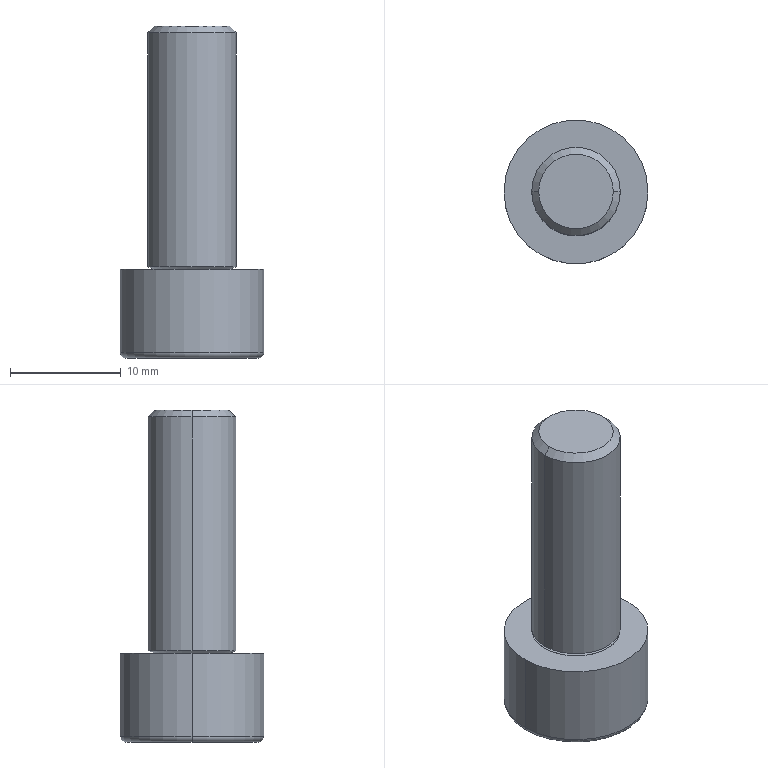Part | SolidWorks | features Attribute 1, Cut 1, Revolution 1 | 1 solid | 27 faces | box 13 x 13 x 30 mm | volume 2066 mm3 | plane 11 | torus 6 | cylinder 6 | cone 4 | commonest cylinder face diameters 8 x4 13 x2
STEP:
#1=CARTESIAN_POINT('',(-3.488,0.,0.01));
#2=VERTEX_POINT('',#1);
#3=CARTESIAN_POINT('',(-3.468,0.,0.03));
#4=VERTEX_POINT('',#3);
#5=CARTESIAN_POINT('',(-3.488,0.,0.03));
#6=DIRECTION('',(0.,-1.,0.));
#7=DIRECTION('',(0.,0.,-1.));
#8=AXIS2_PLACEMENT_3D('',#5,#6,#7);
#9=CIRCLE('',#8,0.02);
#10=EDGE_CURVE('',#2,#4,#9,.T.);
#11=ORIENTED_EDGE('',*,*,#10,.T.);
#12=CARTESIAN_POINT('',(3.468,0.,0.03));
#13=VERTEX_POINT('',#12);
#14=CARTESIAN_POINT('',(0.,0.,0.03));
#15=DIRECTION('',(0.,0.,-1.));
#16=DIRECTION('',(-1.,0.,0.));
#17=AXIS2_PLACEMENT_3D('',#14,#15,#16);
#18=CIRCLE('',#17,3.468);
#19=EDGE_CURVE('',#4,#13,#18,.T.);
#20=ORIENTED_EDGE('',*,*,#19,.T.);
#21=CARTESIAN_POINT('',(3.488,0.,0.01));
#22=VERTEX_POINT('',#21);
#23=CARTESIAN_POINT('',(3.488,0.,0.03));
#24=DIRECTION('',(0.,1.,0.));
#25=DIRECTION('',(-1.,0.,0.));
#26=AXIS2_PLACEMENT_3D('',#23,#24,#25);
#27=CIRCLE('',#26,0.02);
#28=EDGE_CURVE('',#22,#13,#27,.T.);
#29=ORIENTED_EDGE('',*,*,#28,.F.);
#30=CARTESIAN_POINT('',(0.,0.,0.01));
#31=DIRECTION('',(0.,0.,-1.));
#32=DIRECTION('',(-1.,0.,0.));
#33=AXIS2_PLACEMENT_3D('',#30,#31,#32);
#34=CIRCLE('',#33,3.488);
#35=EDGE_CURVE('',#2,#22,#34,.T.);
#36=ORIENTED_EDGE('',*,*,#35,.F.);
#37=EDGE_LOOP('',(#11,#20,#29,#36));
#38=FACE_OUTER_BOUND('',#37,.T.);
#39=CARTESIAN_POINT('',(0.,0.,0.03));
#40=DIRECTION('',(0.,0.,-1.));
#41=DIRECTION('',(-1.,0.,0.));
#42=AXIS2_PLACEMENT_3D('',#39,#40,#41);
#43=TOROIDAL_SURFACE('',#42,3.488,0.02);
#44=ADVANCED_FACE('',(#38),#43,.F.);
#45=ORIENTED_EDGE('',*,*,#28,.T.);
#46=CARTESIAN_POINT('',(0.,0.,0.03));
#47=DIRECTION('',(0.,0.,-1.));
#48=DIRECTION('',(-1.,0.,0.));
#49=AXIS2_PLACEMENT_3D('',#46,#47,#48);
#50=CIRCLE('',#49,3.468);
#51=EDGE_CURVE('',#13,#4,#50,.T.);
#52=ORIENTED_EDGE('',*,*,#51,.T.);
#53=ORIENTED_EDGE('',*,*,#10,.F.);
#54=CARTESIAN_POINT('',(0.,0.,0.01));
#55=DIRECTION('',(0.,0.,-1.));
#56=DIRECTION('',(-1.,0.,0.));
#57=AXIS2_PLACEMENT_3D('',#54,#55,#56);
#58=CIRCLE('',#57,3.488);
#59=EDGE_CURVE('',#22,#2,#58,.T.);
#60=ORIENTED_EDGE('',*,*,#59,.F.);
#61=EDGE_LOOP('',(#45,#52,#53,#60));
#62=FACE_OUTER_BOUND('',#61,.T.);
#63=CARTESIAN_POINT('',(0.,0.,0.03));
#64=DIRECTION('',(0.,0.,-1.));
#65=DIRECTION('',(-1.,0.,0.));
#66=AXIS2_PLACEMENT_3D('',#63,#64,#65);
#67=TOROIDAL_SURFACE('',#66,3.488,0.02);
#68=ADVANCED_FACE('',(#62),#67,.F.);
#69=CARTESIAN_POINT('',(-3.375,0.,22.));
#70=VERTEX_POINT('',#69);
#71=CARTESIAN_POINT('',(3.375,0.,22.));
#72=VERTEX_POINT('',#71);
#73=CARTESIAN_POINT('',(0.,0.,22.));
#74=DIRECTION('',(0.,0.,-1.));
#75=DIRECTION('',(-1.,0.,0.));
#76=AXIS2_PLACEMENT_3D('',#73,#74,#75);
#77=CIRCLE('',#76,3.375);
#78=EDGE_CURVE('',#70,#72,#77,.T.);
#79=ORIENTED_EDGE('',*,*,#78,.T.);
#80=CARTESIAN_POINT('',(4.,0.,21.375));
#81=VERTEX_POINT('',#80);
#82=CARTESIAN_POINT('',(3.375,0.,22.));
#83=DIRECTION('',(0.7071,0.,-0.7071));
#84=VECTOR('',#83,1000.);
#85=LINE('',#82,#84);
#86=EDGE_CURVE('',#72,#81,#85,.T.);
#87=ORIENTED_EDGE('',*,*,#86,.T.);
#88=CARTESIAN_POINT('',(-4.,0.,21.375));
#89=VERTEX_POINT('',#88);
#90=CARTESIAN_POINT('',(0.,0.,21.375));
#91=DIRECTION('',(0.,0.,-1.));
#92=DIRECTION('',(-1.,0.,0.));
#93=AXIS2_PLACEMENT_3D('',#90,#91,#92);
#94=CIRCLE('',#93,4.);
#95=EDGE_CURVE('',#89,#81,#94,.T.);
#96=ORIENTED_EDGE('',*,*,#95,.F.);
#97=CARTESIAN_POINT('',(-3.375,0.,22.));
#98=DIRECTION('',(-0.7071,0.,-0.7071));
#99=VECTOR('',#98,1000.);
#100=LINE('',#97,#99);
#101=EDGE_CURVE('',#70,#89,#100,.T.);
#102=ORIENTED_EDGE('',*,*,#101,.F.);
#103=EDGE_LOOP('',(#79,#87,#96,#102));
#104=FACE_OUTER_BOUND('',#103,.T.);
#105=CARTESIAN_POINT('',(0.,0.,22.));
#106=DIRECTION('',(0.,0.,-1.));
#107=DIRECTION('',(-1.,0.,0.));
#108=AXIS2_PLACEMENT_3D('',#105,#106,#107);
#109=CONICAL_SURFACE('',#108,3.375,0.7854);
#110=ADVANCED_FACE('',(#104),#109,.T.);
#111=ORIENTED_EDGE('',*,*,#95,.T.);
#112=CARTESIAN_POINT('',(4.,0.,0.2375));
#113=VERTEX_POINT('',#112);
#114=CARTESIAN_POINT('',(4.,0.,-10.585));
#115=DIRECTION('',(0.,0.,-1.));
#116=VECTOR('',#115,1000.);
#117=LINE('',#114,#116);
#118=EDGE_CURVE('',#81,#113,#117,.T.);
#119=ORIENTED_EDGE('',*,*,#118,.T.);
#120=CARTESIAN_POINT('',(-4.,0.,0.2375));
#121=VERTEX_POINT('',#120);
#122=CARTESIAN_POINT('',(0.,0.,0.2375));
#123=DIRECTION('',(0.,0.,-1.));
#124=DIRECTION('',(-1.,0.,0.));
#125=AXIS2_PLACEMENT_3D('',#122,#123,#124);
#126=CIRCLE('',#125,4.);
#127=EDGE_CURVE('',#121,#113,#126,.T.);
#128=ORIENTED_EDGE('',*,*,#127,.F.);
#129=CARTESIAN_POINT('',(-4.,0.,-10.585));
#130=DIRECTION('',(0.,0.,-1.));
#131=VECTOR('',#130,1000.);
#132=LINE('',#129,#131);
#133=EDGE_CURVE('',#89,#121,#132,.T.);
#134=ORIENTED_EDGE('',*,*,#133,.F.);
#135=EDGE_LOOP('',(#111,#119,#128,#134));
#136=FACE_OUTER_BOUND('',#135,.T.);
#137=CARTESIAN_POINT('',(0.,0.,-10.585));
#138=DIRECTION('',(0.,0.,-1.));
#139=DIRECTION('',(-1.,0.,0.));
#140=AXIS2_PLACEMENT_3D('',#137,#138,#139);
#141=CYLINDRICAL_SURFACE('',#140,4.);
#142=ADVANCED_FACE('',(#136),#141,.T.);
#143=CARTESIAN_POINT('',(-3.482,0.,0.04879));
#144=VERTEX_POINT('',#143);
#145=CARTESIAN_POINT('',(3.482,0.,0.04879));
#146=VERTEX_POINT('',#145);
#147=CARTESIAN_POINT('',(0.,0.,0.04879));
#148=DIRECTION('',(0.,0.,-1.));
#149=DIRECTION('',(-1.,0.,0.));
#150=AXIS2_PLACEMENT_3D('',#147,#148,#149);
#151=CIRCLE('',#150,3.482);
#152=EDGE_CURVE('',#144,#146,#151,.T.);
#153=ORIENTED_EDGE('',*,*,#152,.F.);
#154=CARTESIAN_POINT('',(-4.,0.,0.2375));
#155=DIRECTION('',(-0.9397,0.,0.342));
#156=VECTOR('',#155,1000.);
#157=LINE('',#154,#156);
#158=EDGE_CURVE('',#144,#121,#157,.T.);
#159=ORIENTED_EDGE('',*,*,#158,.T.);
#160=ORIENTED_EDGE('',*,*,#127,.T.);
#161=CARTESIAN_POINT('',(4.,0.,0.2375));
#162=DIRECTION('',(0.9397,0.,0.342));
#163=VECTOR('',#162,1000.);
#164=LINE('',#161,#163);
#165=EDGE_CURVE('',#146,#113,#164,.T.);
#166=ORIENTED_EDGE('',*,*,#165,.F.);
#167=EDGE_LOOP('',(#153,#159,#160,#166));
#168=FACE_OUTER_BOUND('',#167,.T.);
#169=CARTESIAN_POINT('',(0.,0.,0.2375));
#170=DIRECTION('',(0.,0.,1.));
#171=DIRECTION('',(1.,0.,0.));
#172=AXIS2_PLACEMENT_3D('',#169,#170,#171);
#173=CONICAL_SURFACE('',#172,4.,1.222);
#174=ADVANCED_FACE('',(#168),#173,.T.);
#175=ORIENTED_EDGE('',*,*,#51,.F.);
#176=CARTESIAN_POINT('',(3.488,0.,0.03));
#177=DIRECTION('',(0.,1.,0.));
#178=DIRECTION('',(-1.,0.,0.));
#179=AXIS2_PLACEMENT_3D('',#176,#177,#178);
#180=CIRCLE('',#179,0.02);
#181=EDGE_CURVE('',#13,#146,#180,.T.);
#182=ORIENTED_EDGE('',*,*,#181,.T.);
#183=CARTESIAN_POINT('',(0.,0.,0.04879));
#184=DIRECTION('',(0.,0.,-1.));
#185=DIRECTION('',(-1.,0.,0.));
#186=AXIS2_PLACEMENT_3D('',#183,#184,#185);
#187=CIRCLE('',#186,3.482);
#188=EDGE_CURVE('',#146,#144,#187,.T.);
#189=ORIENTED_EDGE('',*,*,#188,.T.);
#190=CARTESIAN_POINT('',(-3.488,0.,0.03));
#191=DIRECTION('',(0.,-1.,0.));
#192=DIRECTION('',(0.,0.,-1.));
#193=AXIS2_PLACEMENT_3D('',#190,#191,#192);
#194=CIRCLE('',#193,0.02);
#195=EDGE_CURVE('',#4,#144,#194,.T.);
#196=ORIENTED_EDGE('',*,*,#195,.F.);
#197=EDGE_LOOP('',(#175,#182,#189,#196));
#198=FACE_OUTER_BOUND('',#197,.T.);
#199=CARTESIAN_POINT('',(0.,0.,0.03));
#200=DIRECTION('',(0.,0.,-1.));
#201=DIRECTION('',(-1.,0.,0.));
#202=AXIS2_PLACEMENT_3D('',#199,#200,#201);
#203=TOROIDAL_SURFACE('',#202,3.488,0.02);
#204=ADVANCED_FACE('',(#198),#203,.F.);
#205=CARTESIAN_POINT('',(-4.,0.,0.01));
#206=VERTEX_POINT('',#205);
#207=CARTESIAN_POINT('',(4.,0.,0.01));
#208=VERTEX_POINT('',#207);
#209=CARTESIAN_POINT('',(0.,0.,0.01));
#210=DIRECTION('',(0.,0.,-1.));
#211=DIRECTION('',(-1.,0.,0.));
#212=AXIS2_PLACEMENT_3D('',#209,#210,#211);
#213=CIRCLE('',#212,4.);
#214=EDGE_CURVE('',#206,#208,#213,.T.);
#215=ORIENTED_EDGE('',*,*,#214,.T.);
#216=CARTESIAN_POINT('',(4.,0.,0.));
#217=VERTEX_POINT('',#216);
#218=CARTESIAN_POINT('',(4.,0.,-10.585));
#219=DIRECTION('',(0.,0.,-1.));
#220=VECTOR('',#219,1000.);
#221=LINE('',#218,#220);
#222=EDGE_CURVE('',#208,#217,#221,.T.);
#223=ORIENTED_EDGE('',*,*,#222,.T.);
#224=CARTESIAN_POINT('',(-4.,0.,0.));
#225=VERTEX_POINT('',#224);
#226=CARTESIAN_POINT('',(0.,0.,0.));
#227=DIRECTION('',(0.,0.,-1.));
#228=DIRECTION('',(-1.,0.,0.));
#229=AXIS2_PLACEMENT_3D('',#226,#227,#228);
#230=CIRCLE('',#229,4.);
#231=EDGE_CURVE('',#225,#217,#230,.T.);
#232=ORIENTED_EDGE('',*,*,#231,.F.);
#233=CARTESIAN_POINT('',(-4.,0.,-10.585));
#234=DIRECTION('',(0.,0.,-1.));
#235=VECTOR('',#234,1000.);
#236=LINE('',#233,#235);
#237=EDGE_CURVE('',#206,#225,#236,.T.);
#238=ORIENTED_EDGE('',*,*,#237,.F.);
#239=EDGE_LOOP('',(#215,#223,#232,#238));
#240=FACE_OUTER_BOUND('',#239,.T.);
#241=CARTESIAN_POINT('',(0.,0.,-10.585));
#242=DIRECTION('',(0.,0.,-1.));
#243=DIRECTION('',(-1.,0.,0.));
#244=AXIS2_PLACEMENT_3D('',#241,#242,#243);
#245=CYLINDRICAL_SURFACE('',#244,4.);
#246=ADVANCED_FACE('',(#240),#245,.T.);
#247=CARTESIAN_POINT('',(-6.5,0.,0.));
#248=VERTEX_POINT('',#247);
#249=CARTESIAN_POINT('',(6.5,0.,0.));
#250=VERTEX_POINT('',#249);
#251=CARTESIAN_POINT('',(0.,0.,0.));
#252=DIRECTION('',(0.,0.,-1.));
#253=DIRECTION('',(-1.,0.,0.));
#254=AXIS2_PLACEMENT_3D('',#251,#252,#253);
#255=CIRCLE('',#254,6.5);
#256=EDGE_CURVE('',#248,#250,#255,.T.);
#257=ORIENTED_EDGE('',*,*,#256,.T.);
#258=CARTESIAN_POINT('',(6.5,0.,-7.5));
#259=VERTEX_POINT('',#258);
#260=CARTESIAN_POINT('',(6.5,0.,-10.585));
#261=DIRECTION('',(0.,0.,-1.));
#262=VECTOR('',#261,1000.);
#263=LINE('',#260,#262);
#264=EDGE_CURVE('',#250,#259,#263,.T.);
#265=ORIENTED_EDGE('',*,*,#264,.T.);
#266=CARTESIAN_POINT('',(-6.5,0.,-7.5));
#267=VERTEX_POINT('',#266);
#268=CARTESIAN_POINT('',(0.,0.,-7.5));
#269=DIRECTION('',(0.,0.,-1.));
#270=DIRECTION('',(-1.,0.,0.));
#271=AXIS2_PLACEMENT_3D('',#268,#269,#270);
#272=CIRCLE('',#271,6.5);
#273=EDGE_CURVE('',#267,#259,#272,.T.);
#274=ORIENTED_EDGE('',*,*,#273,.F.);
#275=CARTESIAN_POINT('',(-6.5,0.,-10.585));
#276=DIRECTION('',(0.,0.,-1.));
#277=VECTOR('',#276,1000.);
#278=LINE('',#275,#277);
#279=EDGE_CURVE('',#248,#267,#278,.T.);
#280=ORIENTED_EDGE('',*,*,#279,.F.);
#281=EDGE_LOOP('',(#257,#265,#274,#280));
#282=FACE_OUTER_BOUND('',#281,.T.);
#283=CARTESIAN_POINT('',(0.,0.,-10.585));
#284=DIRECTION('',(0.,0.,-1.));
#285=DIRECTION('',(-1.,0.,0.));
#286=AXIS2_PLACEMENT_3D('',#283,#284,#285);
#287=CYLINDRICAL_SURFACE('',#286,6.5);
#288=ADVANCED_FACE('',(#282),#287,.T.);
#289=ORIENTED_EDGE('',*,*,#273,.T.);
#290=CARTESIAN_POINT('',(6.,0.,-8.));
#291=VERTEX_POINT('',#290);
#292=CARTESIAN_POINT('',(6.,0.,-7.5));
#293=DIRECTION('',(0.,1.,0.));
#294=DIRECTION('',(-1.,0.,0.));
#295=AXIS2_PLACEMENT_3D('',#292,#293,#294);
#296=CIRCLE('',#295,0.5);
#297=EDGE_CURVE('',#259,#291,#296,.T.);
#298=ORIENTED_EDGE('',*,*,#297,.T.);
#299=CARTESIAN_POINT('',(-6.,0.,-8.));
#300=VERTEX_POINT('',#299);
#301=CARTESIAN_POINT('',(0.,0.,-8.));
#302=DIRECTION('',(0.,0.,-1.));
#303=DIRECTION('',(-1.,0.,0.));
#304=AXIS2_PLACEMENT_3D('',#301,#302,#303);
#305=CIRCLE('',#304,6.);
#306=EDGE_CURVE('',#300,#291,#305,.T.);
#307=ORIENTED_EDGE('',*,*,#306,.F.);
#308=CARTESIAN_POINT('',(-6.,0.,-7.5));
#309=DIRECTION('',(0.,-1.,0.));
#310=DIRECTION('',(0.,0.,-1.));
#311=AXIS2_PLACEMENT_3D('',#308,#309,#310);
#312=CIRCLE('',#311,0.5);
#313=EDGE_CURVE('',#267,#300,#312,.T.);
#314=ORIENTED_EDGE('',*,*,#313,.F.);
#315=EDGE_LOOP('',(#289,#298,#307,#314));
#316=FACE_OUTER_BOUND('',#315,.T.);
#317=CARTESIAN_POINT('',(0.,0.,-7.5));
#318=DIRECTION('',(0.,0.,-1.));
#319=DIRECTION('',(-1.,0.,0.));
#320=AXIS2_PLACEMENT_3D('',#317,#318,#319);
#321=TOROIDAL_SURFACE('',#320,6.,0.5);
#322=ADVANCED_FACE('',(#316),#321,.T.);
#323=ORIENTED_EDGE('',*,*,#297,.F.);
#324=CARTESIAN_POINT('',(0.,0.,-7.5));
#325=DIRECTION('',(0.,0.,-1.));
#326=DIRECTION('',(-1.,0.,0.));
#327=AXIS2_PLACEMENT_3D('',#324,#325,#326);
#328=CIRCLE('',#327,6.5);
#329=EDGE_CURVE('',#259,#267,#328,.T.);
#330=ORIENTED_EDGE('',*,*,#329,.T.);
#331=ORIENTED_EDGE('',*,*,#313,.T.);
#332=CARTESIAN_POINT('',(0.,0.,-8.));
#333=DIRECTION('',(0.,0.,-1.));
#334=DIRECTION('',(-1.,0.,0.));
#335=AXIS2_PLACEMENT_3D('',#332,#333,#334);
#336=CIRCLE('',#335,6.);
#337=EDGE_CURVE('',#291,#300,#336,.T.);
#338=ORIENTED_EDGE('',*,*,#337,.F.);
#339=EDGE_LOOP('',(#323,#330,#331,#338));
#340=FACE_OUTER_BOUND('',#339,.T.);
#341=CARTESIAN_POINT('',(0.,0.,-7.5));
#342=DIRECTION('',(0.,0.,-1.));
#343=DIRECTION('',(-1.,0.,0.));
#344=AXIS2_PLACEMENT_3D('',#341,#342,#343);
#345=TOROIDAL_SURFACE('',#344,6.,0.5);
#346=ADVANCED_FACE('',(#340),#345,.T.);
#347=ORIENTED_EDGE('',*,*,#264,.F.);
#348=CARTESIAN_POINT('',(0.,0.,0.));
#349=DIRECTION('',(0.,0.,-1.));
#350=DIRECTION('',(-1.,0.,0.));
#351=AXIS2_PLACEMENT_3D('',#348,#349,#350);
#352=CIRCLE('',#351,6.5);
#353=EDGE_CURVE('',#250,#248,#352,.T.);
#354=ORIENTED_EDGE('',*,*,#353,.T.);
#355=ORIENTED_EDGE('',*,*,#279,.T.);
#356=ORIENTED_EDGE('',*,*,#329,.F.);
#357=EDGE_LOOP('',(#347,#354,#355,#356));
#358=FACE_OUTER_BOUND('',#357,.T.);
#359=CARTESIAN_POINT('',(0.,0.,-10.585));
#360=DIRECTION('',(0.,0.,-1.));
#361=DIRECTION('',(-1.,0.,0.));
#362=AXIS2_PLACEMENT_3D('',#359,#360,#361);
#363=CYLINDRICAL_SURFACE('',#362,6.5);
#364=ADVANCED_FACE('',(#358),#363,.T.);
#365=ORIENTED_EDGE('',*,*,#256,.F.);
#366=ORIENTED_EDGE('',*,*,#353,.F.);
#367=EDGE_LOOP('',(#365,#366));
#368=FACE_OUTER_BOUND('',#367,.T.);
#369=ORIENTED_EDGE('',*,*,#231,.T.);
#370=CARTESIAN_POINT('',(0.,0.,0.));
#371=DIRECTION('',(0.,0.,-1.));
#372=DIRECTION('',(-1.,0.,0.));
#373=AXIS2_PLACEMENT_3D('',#370,#371,#372);
#374=CIRCLE('',#373,4.);
#375=EDGE_CURVE('',#217,#225,#374,.T.);
#376=ORIENTED_EDGE('',*,*,#375,.T.);
#377=EDGE_LOOP('',(#369,#376));
#378=FACE_BOUND('',#377,.T.);
#379=CARTESIAN_POINT('',(-6.5,0.,0.));
#380=DIRECTION('',(0.,0.,-1.));
#381=DIRECTION('',(-1.,0.,0.));
#382=AXIS2_PLACEMENT_3D('',#379,#380,#381);
#383=PLANE('',#382);
#384=ADVANCED_FACE('',(#368,#378),#383,.F.);
#385=ORIENTED_EDGE('',*,*,#222,.F.);
#386=CARTESIAN_POINT('',(0.,0.,0.01));
#387=DIRECTION('',(0.,0.,-1.));
#388=DIRECTION('',(-1.,0.,0.));
#389=AXIS2_PLACEMENT_3D('',#386,#387,#388);
#390=CIRCLE('',#389,4.);
#391=EDGE_CURVE('',#208,#206,#390,.T.);
#392=ORIENTED_EDGE('',*,*,#391,.T.);
#393=ORIENTED_EDGE('',*,*,#237,.T.);
#394=ORIENTED_EDGE('',*,*,#375,.F.);
#395=EDGE_LOOP('',(#385,#392,#393,#394));
#396=FACE_OUTER_BOUND('',#395,.T.);
#397=CARTESIAN_POINT('',(0.,0.,-10.585));
#398=DIRECTION('',(0.,0.,-1.));
#399=DIRECTION('',(-1.,0.,0.));
#400=AXIS2_PLACEMENT_3D('',#397,#398,#399);
#401=CYLINDRICAL_SURFACE('',#400,4.);
#402=ADVANCED_FACE('',(#396),#401,.T.);
#403=ORIENTED_EDGE('',*,*,#214,.F.);
#404=ORIENTED_EDGE('',*,*,#391,.F.);
#405=EDGE_LOOP('',(#403,#404));
#406=FACE_OUTER_BOUND('',#405,.T.);
#407=ORIENTED_EDGE('',*,*,#35,.T.);
#408=ORIENTED_EDGE('',*,*,#59,.T.);
#409=EDGE_LOOP('',(#407,#408));
#410=FACE_BOUND('',#409,.T.);
#411=CARTESIAN_POINT('',(-4.,0.,0.01));
#412=DIRECTION('',(0.,0.,-1.));
#413=DIRECTION('',(-1.,0.,0.));
#414=AXIS2_PLACEMENT_3D('',#411,#412,#413);
#415=PLANE('',#414);
#416=ADVANCED_FACE('',(#406,#410),#415,.F.);
#417=ORIENTED_EDGE('',*,*,#19,.F.);
#418=ORIENTED_EDGE('',*,*,#195,.T.);
#419=ORIENTED_EDGE('',*,*,#152,.T.);
#420=ORIENTED_EDGE('',*,*,#181,.F.);
#421=EDGE_LOOP('',(#417,#418,#419,#420));
#422=FACE_OUTER_BOUND('',#421,.T.);
#423=CARTESIAN_POINT('',(0.,0.,0.03));
#424=DIRECTION('',(0.,0.,-1.));
#425=DIRECTION('',(-1.,0.,0.));
#426=AXIS2_PLACEMENT_3D('',#423,#424,#425);
#427=TOROIDAL_SURFACE('',#426,3.488,0.02);
#428=ADVANCED_FACE('',(#422),#427,.F.);
#429=ORIENTED_EDGE('',*,*,#158,.F.);
#430=ORIENTED_EDGE('',*,*,#188,.F.);
#431=ORIENTED_EDGE('',*,*,#165,.T.);
#432=CARTESIAN_POINT('',(0.,0.,0.2375));
#433=DIRECTION('',(0.,0.,-1.));
#434=DIRECTION('',(-1.,0.,0.));
#435=AXIS2_PLACEMENT_3D('',#432,#433,#434);
#436=CIRCLE('',#435,4.);
#437=EDGE_CURVE('',#113,#121,#436,.T.);
#438=ORIENTED_EDGE('',*,*,#437,.T.);
#439=EDGE_LOOP('',(#429,#430,#431,#438));
#440=FACE_OUTER_BOUND('',#439,.T.);
#441=CARTESIAN_POINT('',(0.,0.,0.2375));
#442=DIRECTION('',(0.,0.,1.));
#443=DIRECTION('',(1.,0.,0.));
#444=AXIS2_PLACEMENT_3D('',#441,#442,#443);
#445=CONICAL_SURFACE('',#444,4.,1.222);
#446=ADVANCED_FACE('',(#440),#445,.T.);
#447=ORIENTED_EDGE('',*,*,#118,.F.);
#448=CARTESIAN_POINT('',(0.,0.,21.375));
#449=DIRECTION('',(0.,0.,-1.));
#450=DIRECTION('',(-1.,0.,0.));
#451=AXIS2_PLACEMENT_3D('',#448,#449,#450);
#452=CIRCLE('',#451,4.);
#453=EDGE_CURVE('',#81,#89,#452,.T.);
#454=ORIENTED_EDGE('',*,*,#453,.T.);
#455=ORIENTED_EDGE('',*,*,#133,.T.);
#456=ORIENTED_EDGE('',*,*,#437,.F.);
#457=EDGE_LOOP('',(#447,#454,#455,#456));
#458=FACE_OUTER_BOUND('',#457,.T.);
#459=CARTESIAN_POINT('',(0.,0.,-10.585));
#460=DIRECTION('',(0.,0.,-1.));
#461=DIRECTION('',(-1.,0.,0.));
#462=AXIS2_PLACEMENT_3D('',#459,#460,#461);
#463=CYLINDRICAL_SURFACE('',#462,4.);
#464=ADVANCED_FACE('',(#458),#463,.T.);
#465=ORIENTED_EDGE('',*,*,#86,.F.);
#466=CARTESIAN_POINT('',(0.,0.,22.));
#467=DIRECTION('',(0.,0.,-1.));
#468=DIRECTION('',(-1.,0.,0.));
#469=AXIS2_PLACEMENT_3D('',#466,#467,#468);
#470=CIRCLE('',#469,3.375);
#471=EDGE_CURVE('',#72,#70,#470,.T.);
#472=ORIENTED_EDGE('',*,*,#471,.T.);
#473=ORIENTED_EDGE('',*,*,#101,.T.);
#474=ORIENTED_EDGE('',*,*,#453,.F.);
#475=EDGE_LOOP('',(#465,#472,#473,#474));
#476=FACE_OUTER_BOUND('',#475,.T.);
#477=CARTESIAN_POINT('',(0.,0.,22.));
#478=DIRECTION('',(0.,0.,-1.));
#479=DIRECTION('',(-1.,0.,0.));
#480=AXIS2_PLACEMENT_3D('',#477,#478,#479);
#481=CONICAL_SURFACE('',#480,3.375,0.7854);
#482=ADVANCED_FACE('',(#476),#481,.T.);
#483=ORIENTED_EDGE('',*,*,#78,.F.);
#484=ORIENTED_EDGE('',*,*,#471,.F.);
#485=EDGE_LOOP('',(#483,#484));
#486=FACE_OUTER_BOUND('',#485,.T.);
#487=CARTESIAN_POINT('',(-3.375,0.,22.));
#488=DIRECTION('',(0.,0.,-1.));
#489=DIRECTION('',(-1.,0.,0.));
#490=AXIS2_PLACEMENT_3D('',#487,#488,#489);
#491=PLANE('',#490);
#492=ADVANCED_FACE('',(#486),#491,.F.);
#493=CARTESIAN_POINT('',(3.464,0.,-8.));
#494=VERTEX_POINT('',#493);
#495=CARTESIAN_POINT('',(1.732,-3.,-8.));
#496=VERTEX_POINT('',#495);
#497=CARTESIAN_POINT('',(3.464,0.,-8.));
#498=DIRECTION('',(-0.5,-0.866,0.));
#499=VECTOR('',#498,1000.);
#500=LINE('',#497,#499);
#501=EDGE_CURVE('',#494,#496,#500,.T.);
#502=ORIENTED_EDGE('',*,*,#501,.F.);
#503=CARTESIAN_POINT('',(1.732,3.,-8.));
#504=VERTEX_POINT('',#503);
#505=CARTESIAN_POINT('',(1.732,3.,-8.));
#506=DIRECTION('',(0.5,-0.866,0.));
#507=VECTOR('',#506,1000.);
#508=LINE('',#505,#507);
#509=EDGE_CURVE('',#504,#494,#508,.T.);
#510=ORIENTED_EDGE('',*,*,#509,.F.);
#511=CARTESIAN_POINT('',(-1.732,3.,-8.));
#512=VERTEX_POINT('',#511);
#513=CARTESIAN_POINT('',(-1.732,3.,-8.));
#514=DIRECTION('',(1.,0.,0.));
#515=VECTOR('',#514,1000.);
#516=LINE('',#513,#515);
#517=EDGE_CURVE('',#512,#504,#516,.T.);
#518=ORIENTED_EDGE('',*,*,#517,.F.);
#519=CARTESIAN_POINT('',(-3.464,0.,-8.));
#520=VERTEX_POINT('',#519);
#521=CARTESIAN_POINT('',(-3.464,0.,-8.));
#522=DIRECTION('',(0.5,0.866,0.));
#523=VECTOR('',#522,1000.);
#524=LINE('',#521,#523);
#525=EDGE_CURVE('',#520,#512,#524,.T.);
#526=ORIENTED_EDGE('',*,*,#525,.F.);
#527=CARTESIAN_POINT('',(-1.732,-3.,-8.));
#528=VERTEX_POINT('',#527);
#529=CARTESIAN_POINT('',(-1.732,-3.,-8.));
#530=DIRECTION('',(-0.5,0.866,0.));
#531=VECTOR('',#530,1000.);
#532=LINE('',#529,#531);
#533=EDGE_CURVE('',#528,#520,#532,.T.);
#534=ORIENTED_EDGE('',*,*,#533,.F.);
#535=CARTESIAN_POINT('',(1.732,-3.,-8.));
#536=DIRECTION('',(-1.,0.,0.));
#537=VECTOR('',#536,1000.);
#538=LINE('',#535,#537);
#539=EDGE_CURVE('',#496,#528,#538,.T.);
#540=ORIENTED_EDGE('',*,*,#539,.F.);
#541=EDGE_LOOP('',(#502,#510,#518,#526,#534,#540));
#542=FACE_BOUND('',#541,.T.);
#543=ORIENTED_EDGE('',*,*,#306,.T.);
#544=ORIENTED_EDGE('',*,*,#337,.T.);
#545=EDGE_LOOP('',(#543,#544));
#546=FACE_OUTER_BOUND('',#545,.T.);
#547=CARTESIAN_POINT('',(0.,0.,-8.));
#548=DIRECTION('',(0.,0.,1.));
#549=DIRECTION('',(1.,0.,0.));
#550=AXIS2_PLACEMENT_3D('',#547,#548,#549);
#551=PLANE('',#550);
#552=ADVANCED_FACE('',(#542,#546),#551,.F.);
#553=ORIENTED_EDGE('',*,*,#509,.T.);
#554=CARTESIAN_POINT('',(3.464,0.,-5.));
#555=VERTEX_POINT('',#554);
#556=CARTESIAN_POINT('',(3.464,0.,-5.));
#557=DIRECTION('',(0.,0.,-1.));
#558=VECTOR('',#557,1000.);
#559=LINE('',#556,#558);
#560=EDGE_CURVE('',#555,#494,#559,.T.);
#561=ORIENTED_EDGE('',*,*,#560,.F.);
#562=CARTESIAN_POINT('',(1.732,3.,-5.));
#563=VERTEX_POINT('',#562);
#564=CARTESIAN_POINT('',(1.732,3.,-5.));
#565=DIRECTION('',(0.5,-0.866,0.));
#566=VECTOR('',#565,1000.);
#567=LINE('',#564,#566);
#568=EDGE_CURVE('',#563,#555,#567,.T.);
#569=ORIENTED_EDGE('',*,*,#568,.F.);
#570=CARTESIAN_POINT('',(1.732,3.,-5.));
#571=DIRECTION('',(0.,0.,-1.));
#572=VECTOR('',#571,1000.);
#573=LINE('',#570,#572);
#574=EDGE_CURVE('',#563,#504,#573,.T.);
#575=ORIENTED_EDGE('',*,*,#574,.T.);
#576=EDGE_LOOP('',(#553,#561,#569,#575));
#577=FACE_OUTER_BOUND('',#576,.T.);
#578=CARTESIAN_POINT('',(1.732,3.,-5.));
#579=DIRECTION('',(0.866,0.5,0.));
#580=DIRECTION('',(-0.5,0.866,0.));
#581=AXIS2_PLACEMENT_3D('',#578,#579,#580);
#582=PLANE('',#581);
#583=ADVANCED_FACE('',(#577),#582,.F.);
#584=ORIENTED_EDGE('',*,*,#517,.T.);
#585=ORIENTED_EDGE('',*,*,#574,.F.);
#586=CARTESIAN_POINT('',(-1.732,3.,-5.));
#587=VERTEX_POINT('',#586);
#588=CARTESIAN_POINT('',(-1.732,3.,-5.));
#589=DIRECTION('',(1.,0.,0.));
#590=VECTOR('',#589,1000.);
#591=LINE('',#588,#590);
#592=EDGE_CURVE('',#587,#563,#591,.T.);
#593=ORIENTED_EDGE('',*,*,#592,.F.);
#594=CARTESIAN_POINT('',(-1.732,3.,-5.));
#595=DIRECTION('',(0.,0.,-1.));
#596=VECTOR('',#595,1000.);
#597=LINE('',#594,#596);
#598=EDGE_CURVE('',#587,#512,#597,.T.);
#599=ORIENTED_EDGE('',*,*,#598,.T.);
#600=EDGE_LOOP('',(#584,#585,#593,#599));
#601=FACE_OUTER_BOUND('',#600,.T.);
#602=CARTESIAN_POINT('',(-1.732,3.,-5.));
#603=DIRECTION('',(0.,1.,0.));
#604=DIRECTION('',(-1.,0.,0.));
#605=AXIS2_PLACEMENT_3D('',#602,#603,#604);
#606=PLANE('',#605);
#607=ADVANCED_FACE('',(#601),#606,.F.);
#608=ORIENTED_EDGE('',*,*,#525,.T.);
#609=ORIENTED_EDGE('',*,*,#598,.F.);
#610=CARTESIAN_POINT('',(-3.464,0.,-5.));
#611=VERTEX_POINT('',#610);
#612=CARTESIAN_POINT('',(-3.464,0.,-5.));
#613=DIRECTION('',(0.5,0.866,0.));
#614=VECTOR('',#613,1000.);
#615=LINE('',#612,#614);
#616=EDGE_CURVE('',#611,#587,#615,.T.);
#617=ORIENTED_EDGE('',*,*,#616,.F.);
#618=CARTESIAN_POINT('',(-3.464,0.,-5.));
#619=DIRECTION('',(0.,0.,-1.));
#620=VECTOR('',#619,1000.);
#621=LINE('',#618,#620);
#622=EDGE_CURVE('',#611,#520,#621,.T.);
#623=ORIENTED_EDGE('',*,*,#622,.T.);
#624=EDGE_LOOP('',(#608,#609,#617,#623));
#625=FACE_OUTER_BOUND('',#624,.T.);
#626=CARTESIAN_POINT('',(-3.464,0.,-5.));
#627=DIRECTION('',(-0.866,0.5,0.));
#628=DIRECTION('',(-0.5,-0.866,0.));
#629=AXIS2_PLACEMENT_3D('',#626,#627,#628);
#630=PLANE('',#629);
#631=ADVANCED_FACE('',(#625),#630,.F.);
#632=ORIENTED_EDGE('',*,*,#533,.T.);
#633=ORIENTED_EDGE('',*,*,#622,.F.);
#634=CARTESIAN_POINT('',(-1.732,-3.,-5.));
#635=VERTEX_POINT('',#634);
#636=CARTESIAN_POINT('',(-1.732,-3.,-5.));
#637=DIRECTION('',(-0.5,0.866,0.));
#638=VECTOR('',#637,1000.);
#639=LINE('',#636,#638);
#640=EDGE_CURVE('',#635,#611,#639,.T.);
#641=ORIENTED_EDGE('',*,*,#640,.F.);
#642=CARTESIAN_POINT('',(-1.732,-3.,-5.));
#643=DIRECTION('',(0.,0.,-1.));
#644=VECTOR('',#643,1000.);
#645=LINE('',#642,#644);
#646=EDGE_CURVE('',#635,#528,#645,.T.);
#647=ORIENTED_EDGE('',*,*,#646,.T.);
#648=EDGE_LOOP('',(#632,#633,#641,#647));
#649=FACE_OUTER_BOUND('',#648,.T.);
#650=CARTESIAN_POINT('',(-1.732,-3.,-5.));
#651=DIRECTION('',(-0.866,-0.5,0.));
#652=DIRECTION('',(0.5,-0.866,0.));
#653=AXIS2_PLACEMENT_3D('',#650,#651,#652);
#654=PLANE('',#653);
#655=ADVANCED_FACE('',(#649),#654,.F.);
#656=ORIENTED_EDGE('',*,*,#539,.T.);
#657=ORIENTED_EDGE('',*,*,#646,.F.);
#658=CARTESIAN_POINT('',(1.732,-3.,-5.));
#659=VERTEX_POINT('',#658);
#660=CARTESIAN_POINT('',(1.732,-3.,-5.));
#661=DIRECTION('',(-1.,0.,0.));
#662=VECTOR('',#661,1000.);
#663=LINE('',#660,#662);
#664=EDGE_CURVE('',#659,#635,#663,.T.);
#665=ORIENTED_EDGE('',*,*,#664,.F.);
#666=CARTESIAN_POINT('',(1.732,-3.,-5.));
#667=DIRECTION('',(0.,0.,-1.));
#668=VECTOR('',#667,1000.);
#669=LINE('',#666,#668);
#670=EDGE_CURVE('',#659,#496,#669,.T.);
#671=ORIENTED_EDGE('',*,*,#670,.T.);
#672=EDGE_LOOP('',(#656,#657,#665,#671));
#673=FACE_OUTER_BOUND('',#672,.T.);
#674=CARTESIAN_POINT('',(1.732,-3.,-5.));
#675=DIRECTION('',(0.,-1.,0.));
#676=DIRECTION('',(1.,0.,0.));
#677=AXIS2_PLACEMENT_3D('',#674,#675,#676);
#678=PLANE('',#677);
#679=ADVANCED_FACE('',(#673),#678,.F.);
#680=ORIENTED_EDGE('',*,*,#501,.T.);
#681=ORIENTED_EDGE('',*,*,#670,.F.);
#682=CARTESIAN_POINT('',(3.464,0.,-5.));
#683=DIRECTION('',(-0.5,-0.866,0.));
#684=VECTOR('',#683,1000.);
#685=LINE('',#682,#684);
#686=EDGE_CURVE('',#555,#659,#685,.T.);
#687=ORIENTED_EDGE('',*,*,#686,.F.);
#688=ORIENTED_EDGE('',*,*,#560,.T.);
#689=EDGE_LOOP('',(#680,#681,#687,#688));
#690=FACE_OUTER_BOUND('',#689,.T.);
#691=CARTESIAN_POINT('',(3.464,0.,-5.));
#692=DIRECTION('',(0.866,-0.5,0.));
#693=DIRECTION('',(0.5,0.866,0.));
#694=AXIS2_PLACEMENT_3D('',#691,#692,#693);
#695=PLANE('',#694);
#696=ADVANCED_FACE('',(#690),#695,.F.);
#697=ORIENTED_EDGE('',*,*,#568,.T.);
#698=ORIENTED_EDGE('',*,*,#686,.T.);
#699=ORIENTED_EDGE('',*,*,#664,.T.);
#700=ORIENTED_EDGE('',*,*,#640,.T.);
#701=ORIENTED_EDGE('',*,*,#616,.T.);
#702=ORIENTED_EDGE('',*,*,#592,.T.);
#703=EDGE_LOOP('',(#697,#698,#699,#700,#701,#702));
#704=FACE_OUTER_BOUND('',#703,.T.);
#705=CARTESIAN_POINT('',(1.732,3.,-5.));
#706=DIRECTION('',(0.,0.,1.));
#707=DIRECTION('',(1.,0.,0.));
#708=AXIS2_PLACEMENT_3D('',#705,#706,#707);
#709=PLANE('',#708);
#710=ADVANCED_FACE('',(#704),#709,.F.);
#711=CLOSED_SHELL('',(#44,#68,#110,#142,#174,#204,#246,#288,#322,#346,#364,#384,#402,#416,#428,#446,#464,#482,#492,#552,#583,#607,#631,#655,#679,#696,#710));
#712=MANIFOLD_SOLID_BREP('',#711);
#713=CARTESIAN_POINT('',(0.,0.,0.));
#714=DIRECTION('',(0.,0.,1.));
#715=DIRECTION('',(1.,0.,0.));
#716=AXIS2_PLACEMENT_3D('',#713,#714,#715);
#717=(LENGTH_UNIT()NAMED_UNIT(*)SI_UNIT(.MILLI.,.METRE.));
#718=UNCERTAINTY_MEASURE_WITH_UNIT(LENGTH_MEASURE(0.00001),#717,'','');
#719=(NAMED_UNIT(*)PLANE_ANGLE_UNIT()SI_UNIT($,.RADIAN.));
#720=(NAMED_UNIT(*)SI_UNIT($,.STERADIAN.)SOLID_ANGLE_UNIT());
#721=(GEOMETRIC_REPRESENTATION_CONTEXT(3)GLOBAL_UNCERTAINTY_ASSIGNED_CONTEXT((#718))GLOBAL_UNIT_ASSIGNED_CONTEXT((#717,#719,#720))REPRESENTATION_CONTEXT('',''));
#722=ADVANCED_BREP_SHAPE_REPRESENTATION('',(#712,#716),#721);